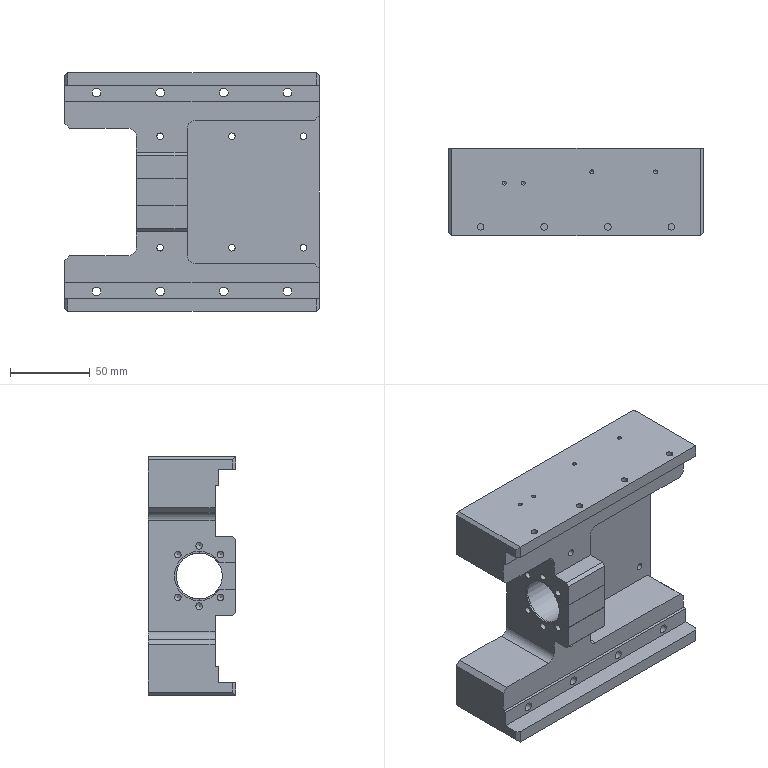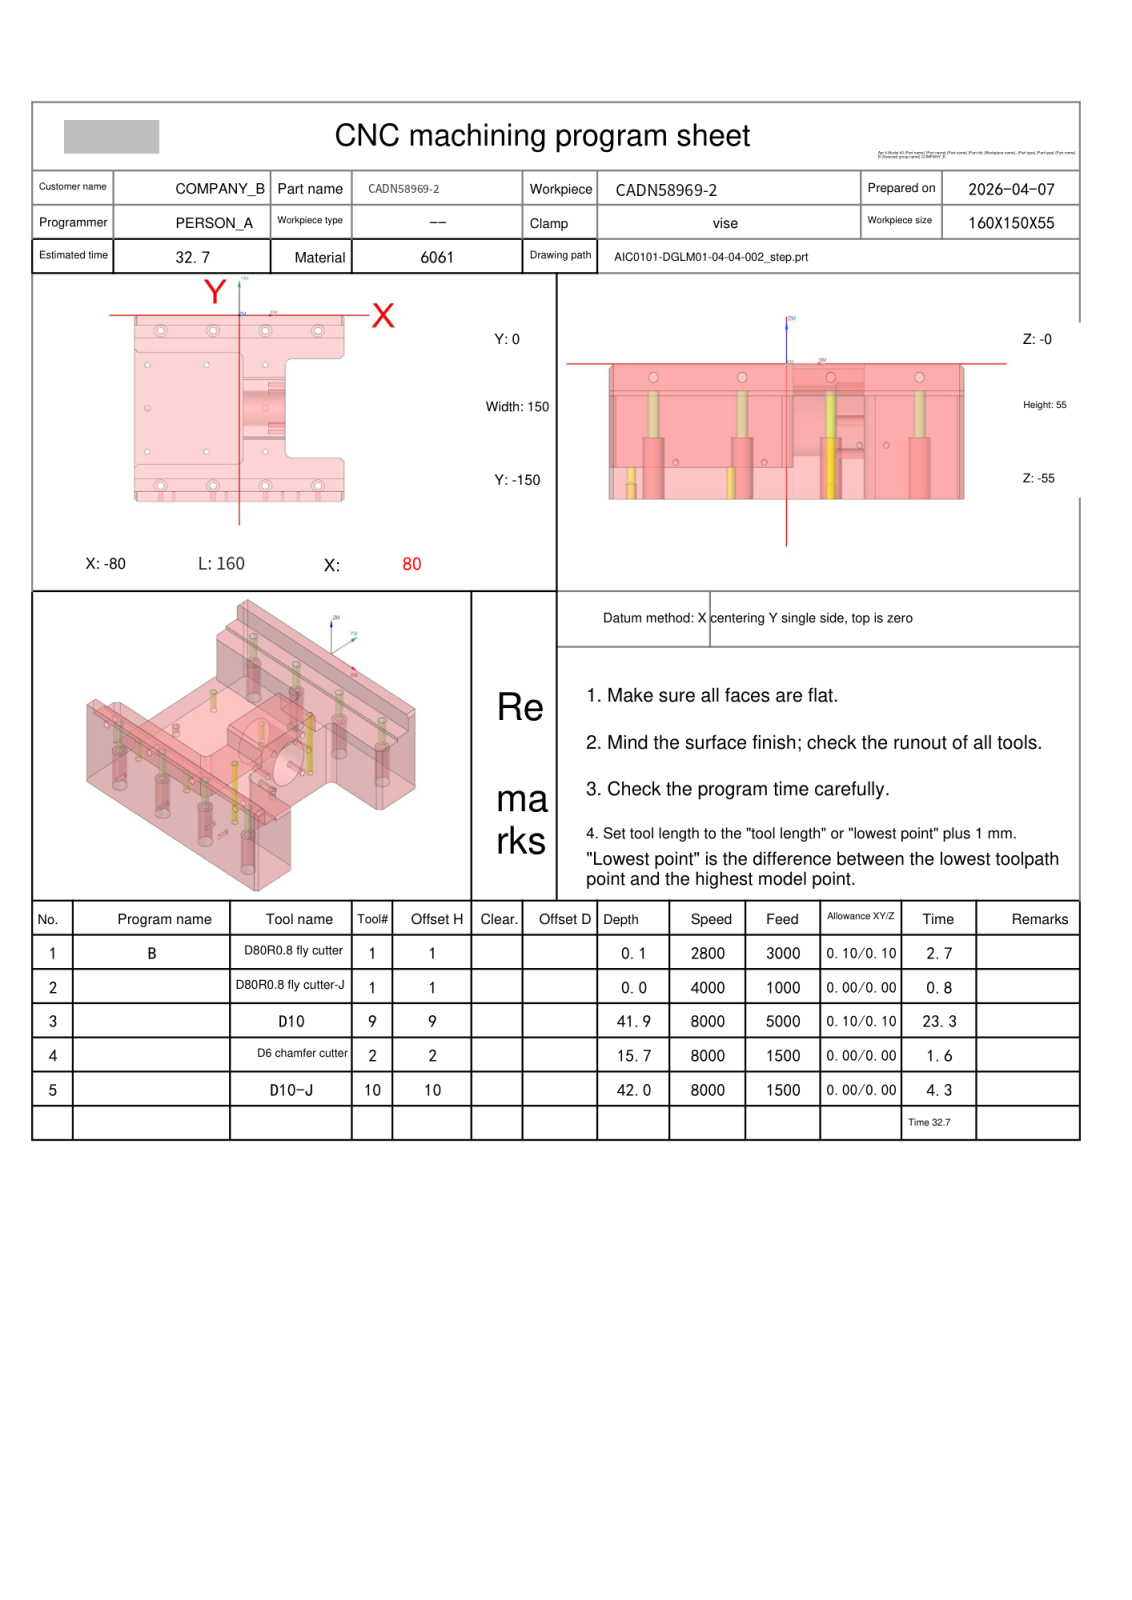NC program | NX | posted by the shop | part box 160 x 55 x 150 mm
Lines 209 to 1320 of 14160:
N3 T09 M06
(D10  D=10. R=0. H=09 ce=0.10 di=0.10)
G00 G90 G54 X-94.5 Y-82. M03 S8000
G43 H09 Z14.5
M08
Z.519
G01 Z-.681 F5000.
X-87.08
G03 X-80.08 Y-75. I0.0 J7.
G01 Y-34.166
X-80.147 Y-34.114
X-80.709 Y-33.618
X-83.001 Y-31.328
Y-29.888
X-80.08 Y-26.967
Y-23.302
X-80.079 Y-22.483
X-80.08 Y-14.353
Y-13.177
G02 X-84.225 Y-10.953 I.109 J5.178
X-85.158 Y-7.649 I5.387 J3.304
X-85.151 Y-7.349 I6.319 J0.0
G01 Y-2.
X-85.127 Y-1.943
X-83.936 Y-.752
X-83.823
Y-8.
G03 X-78.896 Y-13.096 I5.121 J.021
G01 X-78.343 Y-13.168
X-78.169 Y-13.178
X-77.979 Y-13.179
X75.306
X76.197
X77.98
X78.173 Y-13.178
X78.349 Y-13.168
X78.896 Y-13.096
G03 X83.823 Y-8. I-.194 J5.117
G01 Y-.752
X83.932
X85.127 Y-1.954
X85.151 Y-2.01
Y-7.353
X85.13 Y-8.246
G02 X80.08 Y-13.177 I-5.266 J.341
G01 X80.079 Y-22.483
X80.08 Y-23.302
Y-32.
X80.057 Y-32.057
X77.057 Y-35.057
X77. Y-35.08
X40.55
X39.665 Y-35.092
X38.787 Y-35.232
X37.908 Y-35.547
X37.587 Y-35.712
X37.278 Y-35.902
X37.033 Y-36.075
X36.639 Y-36.407
X36.282 Y-36.778
X36.156 Y-36.929
X35.9 Y-37.281
X35.677 Y-37.651
X35.305 Y-38.531
X35.181 Y-39.007
X35.116 Y-39.403
X35.08 Y-40.287
X35.084 Y-44.914
X35.08 Y-46.178
X35.001 Y-46.177
X35.
X34.999
X34.998
X34.92 Y-46.176
X3. Y-46.177
G03 X-2.096 Y-51.087 I.021 J-5.121
G01 X-2.136 Y-51.314
X-2.178 Y-51.857
X-2.179 Y-52.747
Y-97.253
X-2.178 Y-98.149
X-2.135 Y-98.694
X-2.096 Y-98.913
G03 X3. Y-103.823 I5.116 J.211
G01 X33.52
X34.92 Y-103.824
X34.999 Y-103.823
X35.
X35.001
X35.08
Y-105.099
Y-105.264
Y-109.713
X35.134 Y-111.033
X35.279 Y-111.384
X35.307 Y-111.478
X35.407 Y-111.94
X36.157 Y-113.073
X36.28 Y-113.22
X37.035 Y-113.926
X37.277 Y-114.098
X38.341 Y-114.696
X39.665 Y-114.908
X40.55 Y-114.92
X77.
X77.057 Y-114.943
X80.057 Y-117.943
X80.08 Y-118.
Y-121.92
Y-126.701
X80.079 Y-127.517
X80.08 Y-135.647
Y-136.824
G02 X82.733 Y-137.644 I-.158 J-5.213
X85.13 Y-141.758 I-2.811 J-4.393
G01 X85.151 Y-143.539
Y-148.
X85.127 Y-148.057
X83.936 Y-149.248
X83.823
X83.822 Y-141.973
G03 X78.898 Y-136.904 I-5.121 J-.048
G01 X78.343 Y-136.832
X78.169 Y-136.822
X-62.689 Y-136.821
X-77.088
X-77.534
X-77.775
X-78.015 Y-136.822
X-78.173
X-78.349 Y-136.832
X-78.897 Y-136.904
G03 X-83.823 Y-142. I.195 J-5.117
G01 Y-149.248
X-83.932
X-85.127 Y-148.046
X-85.151 Y-147.99
Y-143.538
X-85.13 Y-141.755
G02 X-80.08 Y-136.824 I5.207 J-.281
G01 Y-135.647
Y-123.032
X-83. Y-120.112
Y-118.672
X-80.706 Y-116.378
X-80.143 Y-115.882
X-80.08 Y-115.834
Y-78.014
G02 X-79.662 Y-77.201 I1. J-.001
G01 X-73.498 Y-72.799
G03 X-73.08 Y-71.986 I-.582 J.813
G01 Y-34.166
G03 X-73.83 Y-31.014 I-7. J0.0
G02 X-73.936 Y-30.566 I.894 J.448
X-73.83 Y-30.119 I1. J0.0
G03 X-73.08 Y-26.967 I-6.25 J3.152
G01 X-73.079 Y-21.176
G02 X-72.082 Y-20.179 I1. J-.003
G01 X32.086
G02 X32.78 Y-20.459 I0.0 J-1.
G01 X34.199 Y-21.826
G03 X34.678 Y-22.083 I.694 J.72
G02 X36.641 Y-24.525 I-.537 J-2.442
X34.822 Y-26.93 I-2.5 J0.0
G01 X27.87 Y-28.899
G02 X27.189 Y-28.994 I-.681 J2.405
X24.689 Y-26.494 I0.0 J2.5
X26.507 Y-24.088 I2.5 J0.0
G01 X32.238 Y-22.465
G03 X32.722 Y-22.157 I-.272 J.962
G01 X34.131 Y-20.525
G02 X34.888 Y-20.179 I.757 J-.654
G01 X72.082
G02 X73.079 Y-21.176 I-.003 J-1.
G01 Y-22.486
X73.08 Y-23.306
Y-27.083
G02 X72.083 Y-28.08 I-1. J.003
G01 X40.504
X39.062 Y-28.099
X37.038 Y-28.423
X35.112 Y-29.113
X34.153 Y-29.607
X33.422 Y-30.055
X32.748 Y-30.533
X31.851 Y-31.287
X31.063 Y-32.105
X30.632 Y-32.624
X30.061 Y-33.408
X29.423 Y-34.467
X28.658 Y-36.277
X28.325 Y-37.561
X28.197 Y-38.342
G02 X27.213 Y-39.177 I-.986 J.164
G01 X2.986
G03 X-9.055 Y-50.25 I.035 J-12.121
X-9.114 Y-50.767 I6.999 J-1.07
G01 X-9.156 Y-51.304
G03 X-9.178 Y-51.857 I7.058 J-.553
G01 Y-98.143
G03 X-9.156 Y-98.696 I7.08 J0.0
G01 X-9.114 Y-99.233
G03 X-9.055 Y-99.75 I7.058 J.553
X2.986 Y-110.823 I12.075 J1.048
G01 X27.176
G02 X28.168 Y-111.721 I-.003 J-1.
G03 X28.562 Y-113.441 I6.966 J.688
G01 X28.594 Y-113.549
G03 X29.573 Y-115.809 I6.813 J1.609
G01 X30.534 Y-117.258
X31.179 Y-118.034
X32.6 Y-119.362
X33.526 Y-120.019
X34.908 Y-120.797
G03 X37.234 Y-121.608 I3.433 J6.101
G01 X39.062 Y-121.901
X40.504 Y-121.92
X72.083
G02 X73.08 Y-122.917 I-.003 J-1.
G01 Y-126.696
X73.079 Y-127.514
Y-128.825
G02 X72.082 Y-129.822 I-1. J.003
G01 X34.936
G02 X34.18 Y-129.476 I0.0 J1.
G01 X32.765 Y-127.841
G03 X32.277 Y-127.532 I-.756 J-.654
G01 X26.504 Y-125.921
G02 X24.676 Y-123.513 I.672 J2.408
X27.176 Y-121.013 I2.5 J0.0
X27.848 Y-121.105 I0.0 J-2.5
G01 X34.849 Y-123.059
G02 X36.677 Y-125.467 I-.672 J-2.408
X34.725 Y-127.906 I-2.5 J0.0
G03 X34.249 Y-128.163 I.219 J-.976
G01 X32.823 Y-129.541
G02 X32.128 Y-129.822 I-.695 J.719
G01 X-72.083 Y-129.821
G02 X-73.08 Y-128.824 I.003 J1.
G01 Y-123.032
G03 X-73.83 Y-119.881 I-7. J0.0
G02 X-73.935 Y-119.433 I.894 J.448
X-73.83 Y-118.986 I1. J0.0
G03 X-73.08 Y-115.834 I-6.25 J3.152
G01 Y-78.014
G02 X-72.662 Y-77.201 I1. J0.0
G01 X-66.498 Y-72.799
G03 X-66.08 Y-71.986 I-.582 J.813
G01 Y-34.166
G03 X-66.49 Y-30.803 I-14. J0.0
G02 X-66.518 Y-30.566 I.972 J.237
X-66.49 Y-30.329 I1. J0.0
G03 X-66.126 Y-28.095 I-13.59 J3.363
G02 X-65.132 Y-27.179 I.996 J-.084
G01 X-11.561
G02 X-10.879 Y-27.448 I0.0 J-1.
G01 X-9.582 Y-28.658
G03 X-9.048 Y-28.915 I.682 J.731
G02 X-6.919 Y-31.388 I-.371 J-2.472
X-8.595 Y-33.748 I-2.5 J0.0
G01 X-14.748 Y-35.895
G02 X-15.572 Y-36.035 I-.824 J2.36
X-18.072 Y-33.535 I0.0 J2.5
X-16.396 Y-31.175 I2.5 J0.0
G01 X-11.377 Y-29.423
G03 X-10.938 Y-29.12 I-.329 J.944
G01 X-9.618 Y-27.538
G02 X-8.85 Y-27.179 I.768 J-.641
G01 X23.976
G02 X24.973 Y-28.179 I-.003 J-1.
X24.783 Y-28.765 I-1. J0.0
G01 X24.221 Y-29.535
X23.17 Y-31.283
X23.049 Y-31.57
G02 X22.132 Y-32.177 I-.92 J.393
G01 X2.976
G03 X-16.009 Y-49.431 I.045 J-19.121
X-16.093 Y-50.22 I13.953 J-1.889
G01 X-16.135 Y-50.757
G03 X-16.178 Y-51.857 I14.037 J-1.1
G01 Y-98.143
G03 X-16.135 Y-99.243 I14.08 J0.0
G01 X-16.093 Y-99.78
G03 X-16.009 Y-100.569 I14.037 J1.1
X2.976 Y-117.823 I19.029 J1.867
G01 X22.082
G02 X22.966 Y-118.361 I-.003 J-1.
G03 X23.739 Y-119.678 I12.441 J6.421
G01 X24.796 Y-121.272
G02 X24.961 Y-121.822 I-.835 J-.55
X23.964 Y-122.822 I-1. J0.0
G01 X-8.85
G02 X-9.618 Y-122.462 I0.0 J1.
G01 X-10.938 Y-120.88
G03 X-11.376 Y-120.577 I-.768 J-.641
G01 X-16.395 Y-118.826
G02 X-18.072 Y-116.465 I.824 J2.36
X-15.572 Y-113.965 I2.5 J0.0
X-14.748 Y-114.105 I0.0 J-2.5
G01 X-8.595 Y-116.252
G02 X-6.919 Y-118.612 I-.824 J-2.36
X-9.048 Y-121.085 I-2.5 J0.0
G03 X-9.582 Y-121.343 I.148 J-.989
G01 X-10.879 Y-122.553
G02 X-11.561 Y-122.822 I-.682 J.731
G01 X-65.132 Y-122.821
G02 X-66.125 Y-121.905 I.003 J1.
G03 X-66.49 Y-119.67 I-13.955 J-1.127
G02 X-66.518 Y-119.433 I.972 J.237
X-66.49 Y-119.196 I1. J0.0
G03 X-66.08 Y-115.834 I-13.59 J3.362
G01 Y-115.821
Y-78.014
G02 X-65.662 Y-77.201 I1. J0.0
G01 X-59.498 Y-72.799
G03 X-59.08 Y-71.986 I-.582 J.813
G01 Y-35.175
G02 X-58.084 Y-34.179 I1. J-.004
G01 X-18.786
G02 X-17.79 Y-35.179 I-.004 J-1.
X-17.984 Y-35.77 I-1. J0.0
G03 X-22.963 Y-48.623 I21.004 J-15.528
X-23.071 Y-49.672 I20.907 J-2.697
G01 X-23.114 Y-50.21
G03 X-23.178 Y-51.857 I21.016 J-1.647
G01 Y-98.143
G03 X-23.114 Y-99.79 I21.08 J0.0
G01 X-23.071 Y-100.327
G03 X-22.963 Y-101.377 I21.016 J1.647
X-17.983 Y-114.23 I25.983 J2.675
G02 X-17.79 Y-114.822 I-.806 J-.592
X-18.786 Y-115.822 I-1. J0.0
G01 X-58.084 Y-115.821
G02 X-59.08 Y-114.825 I.004 J1.
G01 Y-78.014
G02 X-58.662 Y-77.201 I1. J0.0
G01 X-52.498 Y-72.799
G03 X-52.08 Y-71.986 I-.582 J.813
G01 Y-42.175
G02 X-51.084 Y-41.179 I1. J-.004
G01 X-29.855
G02 X-28.859 Y-42.179 I-.004 J-1.
X-28.894 Y-42.442 I-1. J0.0
G03 X-29.917 Y-47.817 I31.915 J-8.856
X-30.05 Y-49.125 I27.861 J-3.503
G01 X-30.092 Y-49.663
G03 X-30.178 Y-51.857 I27.994 J-2.194
G01 Y-98.143
G03 X-30.092 Y-100.337 I28.08 J0.0
G01 X-30.05 Y-100.874
G03 X-29.917 Y-102.183 I27.994 J2.195
X-28.894 Y-107.558 I32.937 J3.481
G02 X-28.859 Y-107.822 I-.965 J-.264
X-29.855 Y-108.822 I-1. J0.0
G01 X-51.084 Y-108.821
G02 X-52.08 Y-107.825 I.004 J1.
G01 Y-78.014
G02 X-51.662 Y-77.201 I1. J0.0
G01 X-45.498 Y-72.799
G03 X-45.08 Y-71.986 I-.582 J.813
G01 Y-49.175
G02 X-44.084 Y-48.179 I1. J-.004
G01 X-38.074
G02 X-37.078 Y-49.179 I-.004 J-1.
G01 X-37.081 Y-49.249
G03 X-37.178 Y-51.857 I34.983 J-2.608
G01 Y-98.143
G03 X-37.081 Y-100.751 I35.08 J0.0
G01 X-37.078 Y-100.821
G02 X-38.074 Y-101.821 I-1. J0.0
G01 X-44.084
G02 X-45.08 Y-100.825 I.004 J1.
G01 Y-75.
Y-74.5
G03 X-52.08 Y-67.5 I-7. J0.0
G01 Z.519
G00 Z3.
G01 X-94.5 Y-82. F6000.
G00 Z-.163
G01 Z-1.363 F5000.
X-87.08
G03 X-80.08 Y-75. I0.0 J7.
G01 Y-34.166
X-80.147 Y-34.114
X-80.709 Y-33.618
X-83.001 Y-31.328
Y-29.888
X-80.08 Y-26.967
Y-23.302
X-80.079 Y-22.483
X-80.08 Y-13.177
G02 X-82.321 Y-12.615 I.109 J5.178
X-84.225 Y-10.953 I2.35 J4.615
X-85.158 Y-7.649 I5.387 J3.304
X-85.151 Y-7.349 I6.319 J0.0
G01 Y-2.
X-85.127 Y-1.943
X-84.617 Y-1.433
X-84.504
Y-8.
G03 X-79.383 Y-13.1 I5.121 J.021
G01 X-79.362
X-78.877
X-78.343 Y-13.168
X-78.169 Y-13.178
X-77.979 Y-13.179
X75.306
X76.197
X77.98
X78.173 Y-13.178
X78.349 Y-13.168
X78.877 Y-13.1
X79.362
X79.383
G03 X84.504 Y-8. I0.0 J5.121
G01 Y-1.433
X84.61
X85.127 Y-1.954
X85.151 Y-2.01
Y-7.353
X85.13 Y-8.246
G02 X83. Y-12.149 I-5.266 J.341
X80.08 Y-13.177 I-3.136 J4.244
G01 X80.079 Y-22.483
X80.08 Y-23.302
Y-32.
X80.057 Y-32.057
X77.057 Y-35.057
X77. Y-35.08
X40.55
X39.665 Y-35.092
X38.787 Y-35.232
X37.908 Y-35.547
X37.587 Y-35.712
X37.278 Y-35.902
X37.033 Y-36.075
X36.639 Y-36.407
X36.282 Y-36.778
X36.156 Y-36.929
X35.9 Y-37.281
X35.677 Y-37.651
X35.305 Y-38.531
X35.181 Y-39.007
X35.116 Y-39.403
X35.08 Y-40.287
X35.084 Y-44.914
X35.083 Y-45.496
X35.003
Y-45.495
X34.994 Y-45.496
X34.923 Y-45.495
X3. Y-45.496
G03 X-2.1 Y-50.617 I.021 J-5.121
G01 Y-50.638
Y-51.111
X-2.136 Y-51.314
X-2.178 Y-51.857
X-2.179 Y-52.747
Y-97.253
X-2.178 Y-98.149
X-2.135 Y-98.694
X-2.1 Y-98.889
Y-99.387
G03 X3. Y-104.504 I5.121 J.004
G01 X34.92
X34.999
X35. Y-104.505
X35.001 Y-104.504
X35.08
Y-105.099
Y-105.264
Y-109.713
X35.134 Y-111.033
X35.279 Y-111.384
X35.312 Y-111.504
X35.407 Y-111.94
X36.157 Y-113.073
X36.28 Y-113.22
X37.035 Y-113.926
X37.277 Y-114.098
X38.341 Y-114.696
X39.665 Y-114.908
X40.55 Y-114.92
X77.
X77.057 Y-114.943
X80.057 Y-117.943
X80.08 Y-118.
Y-121.92
Y-126.701
X80.079 Y-127.517
X80.08 Y-136.824
G02 X85.13 Y-141.758 I-.158 J-5.213
G01 X85.151 Y-143.539
Y-148.
X85.127 Y-148.057
X84.617 Y-148.567
X84.504
Y-142.
G03 X79.383 Y-136.9 I-5.121 J-.021
G01 X79.362
X78.879
X78.343 Y-136.832
X78.169 Y-136.822
X-62.689 Y-136.821
X-77.088
X-77.534
X-78.015 Y-136.822
X-78.173
X-78.349 Y-136.832
X-78.879 Y-136.9
X-79.362
X-79.383
G03 X-84.504 Y-142. I0.0 J-5.121
G01 Y-148.567
X-84.61
X-85.127 Y-148.046
X-85.151 Y-147.99
Y-143.538
X-85.13 Y-141.755
G02 X-80.08 Y-136.824 I5.207 J-.281
G01 Y-123.032
X-83. Y-120.112
Y-118.672
X-80.706 Y-116.378
X-80.143 Y-115.882
X-80.08 Y-115.834
Y-78.014
G02 X-79.662 Y-77.201 I1. J0.0
G01 X-73.498 Y-72.799
G03 X-73.08 Y-71.986 I-.582 J.813
G01 Y-34.166
G03 X-73.83 Y-31.014 I-7. J0.0
G02 X-73.936 Y-30.566 I.894 J.447
X-73.83 Y-30.119 I1. J0.0
G03 X-73.08 Y-26.967 I-6.25 J3.152
G01 X-73.079 Y-21.176
G02 X-72.082 Y-20.179 I1. J-.003
G01 X32.086
G02 X32.78 Y-20.459 I0.0 J-1.
G01 X34.199 Y-21.826
G03 X34.678 Y-22.083 I.694 J.72
G02 X36.641 Y-24.525 I-.537 J-2.442
X34.822 Y-26.93 I-2.5 J0.0
G01 X27.87 Y-28.899
G02 X27.189 Y-28.994 I-.681 J2.405
X24.689 Y-26.494 I0.0 J2.5
X26.507 Y-24.088 I2.5 J0.0
G01 X32.238 Y-22.465
G03 X32.722 Y-22.157 I-.272 J.962
G01 X34.131 Y-20.525
G02 X34.888 Y-20.179 I.757 J-.654
G01 X72.082
G02 X73.079 Y-21.176 I-.003 J-1.
G01 Y-22.486
X73.08 Y-23.306
Y-27.083
G02 X72.083 Y-28.08 I-1. J.003
G01 X40.504
X39.062 Y-28.099
X37.038 Y-28.423
X35.112 Y-29.113
X34.153 Y-29.607
X33.422 Y-30.055
X32.748 Y-30.533
X31.851 Y-31.287
X31.063 Y-32.105
X30.632 Y-32.624
X30.061 Y-33.408
X29.423 Y-34.467
X28.658 Y-36.277
X28.325 Y-37.561
X28.309 Y-37.661
G02 X27.325 Y-38.496 I-.986 J.165
G01 X2.986
G03 X-9.1 Y-50.608 I.035 J-12.121
G01 X-9.156 Y-51.303
G03 X-9.178 Y-51.857 I7.058 J-.553
G01 Y-98.143
G03 X-9.156 Y-98.697 I7.08 J0.0
G01 X-9.1 Y-99.392
G03 X2.986 Y-111.504 I12.121 J.009
G01 X27.274
G02 X28.253 Y-112.317 I-.003 J-1.
G03 X28.562 Y-113.441 I6.881 J1.284
G01 X28.594 Y-113.549
G03 X29.573 Y-115.809 I6.813 J1.609
G01 X30.534 Y-117.258
X31.179 Y-118.034
X32.6 Y-119.362
X33.526 Y-120.019
X34.908 Y-120.797
G03 X37.234 Y-121.608 I3.433 J6.101
G01 X39.062 Y-121.901
X40.504 Y-121.92
X72.083
G02 X73.08 Y-122.917 I-.003 J-1.
G01 Y-126.696
X73.079 Y-127.514
Y-128.825
G02 X72.082 Y-129.822 I-1. J.003
G01 X34.936
G02 X34.18 Y-129.476 I0.0 J1.
G01 X32.765 Y-127.841
G03 X32.277 Y-127.532 I-.756 J-.654
G01 X26.504 Y-125.921
G02 X24.676 Y-123.513 I.672 J2.408
X27.176 Y-121.013 I2.5 J0.0
X27.848 Y-121.105 I0.0 J-2.5
G01 X34.849 Y-123.059
G02 X36.677 Y-125.467 I-.672 J-2.408
X34.725 Y-127.906 I-2.5 J0.0
G03 X34.249 Y-128.163 I.219 J-.976
G01 X32.822 Y-129.541
G02 X32.128 Y-129.822 I-.695 J.719
G01 X-62.689 Y-129.821
X-72.083
G02 X-73.08 Y-128.824 I.003 J1.
G01 Y-123.032
G03 X-73.83 Y-119.881 I-7. J0.0
G02 X-73.935 Y-119.433 I.894 J.447
X-73.83 Y-118.986 I1. J0.0
G03 X-73.08 Y-115.834 I-6.25 J3.152
G01 Y-78.014
G02 X-72.662 Y-77.201 I1. J0.0
G01 X-66.498 Y-72.799
G03 X-66.08 Y-71.986 I-.582 J.813
G01 Y-34.166
G03 X-66.49 Y-30.803 I-14. J0.0
G02 X-66.518 Y-30.566 I.972 J.237
X-66.49 Y-30.33 I1. J0.0
G03 X-66.125 Y-28.094 I-13.59 J3.363
G02 X-65.133 Y-27.179 I.996 J-.084
G01 X-12.45
G02 X-11.771 Y-27.444 I0.0 J-1.
G01 X-10.51 Y-28.609
G03 X-9.96 Y-28.866 I.679 J.735
G02 X-7.78 Y-31.346 I-.32 J-2.479
X-9.412 Y-33.691 I-2.5 J0.0
G01 X-15.215 Y-35.837
G02 X-16.082 Y-35.992 I-.867 J2.345
X-18.582 Y-33.492 I0.0 J2.5
X-16.95 Y-31.148 I2.5 J0.0
G01 X-12.254 Y-29.411
G03 X-11.83 Y-29.11 I-.347 J.938
G01 X-10.536 Y-27.542
G02 X-9.765 Y-27.179 I.771 J-.637
G01 X23.976
G02 X24.973 Y-28.179 I-.004 J-1.
X24.783 Y-28.765 I-1. J0.0
G01 X24.221 Y-29.535
X23.332 Y-31.014
G02 X22.48 Y-31.496 I-.855 J.518
G01 X2.976
G03 X-16.097 Y-50.29 I.045 J-19.121
G01 X-16.134 Y-50.747
G03 X-16.178 Y-51.856 I14.036 J-1.11
G01 Y-98.144
G03 X-16.134 Y-99.253 I14.08 J0.0
G01 X-16.097 Y-99.71
G03 X2.976 Y-118.504 I19.118 J.326
G01 X22.457
G02 X23.315 Y-118.997 I-.004 J-1.
G03 X23.739 Y-119.678 I12.092 J7.056
G01 X24.796 Y-121.272
G02 X24.961 Y-121.822 I-.835 J-.55
X23.965 Y-122.822 I-1. J0.0
G01 X-9.765 Y-122.821
G02 X-10.536 Y-122.458 I0.0 J1.
G01 X-11.83 Y-120.89
G03 X-12.254 Y-120.589 I-.771 J-.637
G01 X-16.95 Y-118.852
G02 X-18.582 Y-116.508 I.867 J2.345
X-16.082 Y-114.008 I2.5 J0.0
X-15.215 Y-114.163 I0.0 J-2.5
G01 X-9.412 Y-116.309
G02 X-7.78 Y-118.654 I-.867 J-2.345
X-9.96 Y-121.134 I-2.5 J0.0
G03 X-10.511 Y-121.391 I.128 J-.992
G01 X-11.771 Y-122.556
G02 X-12.45 Y-122.821 I-.679 J.734
G01 X-62.689
X-65.132
G02 X-66.125 Y-121.905 I.003 J1.
G03 X-66.49 Y-119.67 I-13.955 J-1.127
G02 X-66.518 Y-119.433 I.972 J.237
X-66.49 Y-119.197 I1. J0.0
G03 X-66.08 Y-115.834 I-13.59 J3.362
G01 Y-115.821
Y-78.014
G02 X-65.662 Y-77.201 I1. J0.0
G01 X-59.498 Y-72.799
G03 X-59.08 Y-71.986 I-.582 J.813
G01 Y-35.175
G02 X-58.084 Y-34.179 I1. J-.004
G01 X-19.273
G02 X-18.277 Y-35.179 I-.004 J-1.
X-18.453 Y-35.745 I-1. J0.0
G03 X-23.091 Y-49.93 I21.474 J-14.872
G01 X-23.112 Y-50.189
G03 X-23.178 Y-51.856 I21.014 J-1.668
G01 Y-98.144
G03 X-23.112 Y-99.811 I21.08 J.001
G01 X-23.091 Y-100.07
G03 X-18.453 Y-114.255 I26.112 J.686
G02 X-18.277 Y-114.821 I-.824 J-.566
X-19.273 Y-115.821 I-1. J0.0
G01 X-58.084
G02 X-59.08 Y-114.825 I.004 J1.
G01 Y-78.014
G02 X-58.662 Y-77.201 I1. J0.0
G01 X-52.498 Y-72.799
G03 X-52.08 Y-71.986 I-.582 J.813
G01 Y-42.175
G02 X-51.084 Y-41.179 I1. J-.004
G01 X-30.036
G02 X-29.04 Y-42.179 I-.004 J-1.
X-29.07 Y-42.422 I-1. J0.0
G03 X-30.083 Y-49.544 I32.091 J-8.195
G01 X-30.09 Y-49.63
G03 X-30.178 Y-51.856 I27.992 J-2.227
G01 Y-98.144
G03 X-30.083 Y-100.456 I28.08 J.001
X-29.07 Y-107.578 I33.103 J1.072
G02 X-29.04 Y-107.821 I-.97 J-.243
X-30.036 Y-108.821 I-1. J0.0
G01 X-51.084
G02 X-52.08 Y-107.825 I.004 J1.
G01 Y-78.014
G02 X-51.662 Y-77.201 I1. J0.0
G01 X-45.498 Y-72.799
G03 X-45.08 Y-71.986 I-.582 J.813
G01 Y-49.174
G02 X-44.084 Y-48.179 I1. J-.004
G01 X-38.074
G02 X-37.078 Y-49.179 I-.004 J-1.
G01 X-37.081 Y-49.249
G03 X-37.178 Y-51.856 I34.983 J-2.608
G01 Y-98.144
G03 X-37.081 Y-100.751 I35.08 J.001
G01 X-37.079 Y-100.821
G02 X-38.074 Y-101.821 I-1. J0.0
G01 X-44.084
G02 X-45.08 Y-100.825 I.004 J1.
G01 Y-75.
Y-74.5
G03 X-52.08 Y-67.5 I-7. J0.0
G01 Z-.163
G00 Z3.
G01 X-94.5 Y-82. F6000.
G00 Z-.844
G01 Z-2.044 F5000.
X-87.08
G03 X-80.08 Y-75. I0.0 J7.
G01 Y-34.166
X-80.147 Y-34.114
X-80.709 Y-33.618
X-83.001 Y-31.328
Y-29.888
X-80.08 Y-26.967
Y-23.302
X-80.079 Y-22.483
X-80.08 Y-13.177
X-80.059 Y-13.1
X-79.362
X-78.877
X-78.343 Y-13.168
X-78.169 Y-13.178
X-77.979 Y-13.179
X75.306
X76.197
X77.98
X78.173 Y-13.178
X78.349 Y-13.168
X78.877 Y-13.1
X79.404
X80.07
X80.08 Y-13.177
X80.079 Y-22.483
X80.08 Y-23.302
Y-32.
X80.057 Y-32.057
X77.057 Y-35.057
X77. Y-35.08
X40.55
X39.665 Y-35.092
X38.787 Y-35.232
X37.908 Y-35.547
X37.587 Y-35.712
X37.278 Y-35.902
X37.033 Y-36.075
X36.639 Y-36.407
X36.282 Y-36.778
X36.156 Y-36.929
X35.9 Y-37.281
X35.677 Y-37.651
X35.305 Y-38.531
X35.181 Y-39.007
X35.116 Y-39.403
X35.08 Y-40.287
X35.081 Y-44.889
X35.023 Y-44.9
X35.022 Y-44.899
X26.424 Y-44.9
X3.
G03 X-2.1 Y-50. I0.0 J-5.1
G01 Y-51.111
X-2.136 Y-51.314
X-2.178 Y-51.857
X-2.179 Y-52.747
Y-97.253
X-2.178 Y-98.149
X-2.135 Y-98.694
X-2.1 Y-98.889
Y-99.404
Y-100.045
G03 X3. Y-105.1 I5.1 J.045
G01 X34.92
X35.08
Y-105.264
Y-109.713
X35.134 Y-111.033
X35.279 Y-111.384
X35.307 Y-111.478
X35.407 Y-111.94
X36.157 Y-113.073
X36.28 Y-113.22
X37.035 Y-113.926
X37.277 Y-114.098
X38.341 Y-114.696
X39.665 Y-114.908
X40.55 Y-114.92
X77.
X77.057 Y-114.943
X80.057 Y-117.943
X80.08 Y-118.
Y-121.92
Y-126.701
X80.079 Y-127.517
X80.08 Y-136.824
X79.92 Y-136.899
X78.879 Y-136.9
X78.867 Y-136.898
X78.559 Y-136.859
X78.343 Y-136.832
X78.169 Y-136.822
X-62.689 Y-136.821
X-77.088
X-77.311
X-77.534
X-78.173 Y-136.822
X-78.349 Y-136.832
X-78.879 Y-136.9
X-79.363
X-79.404
X-79.92
X-80.08 Y-136.824
Y-123.032
X-83. Y-120.112
Y-118.672
X-80.706 Y-116.378
X-80.143 Y-115.882
X-80.08 Y-115.834
Y-78.014
G02 X-79.662 Y-77.201 I1. J0.0
G01 X-73.498 Y-72.799
G03 X-73.08 Y-71.986 I-.582 J.813
G01 Y-34.166
G03 X-73.83 Y-31.014 I-7. J0.0
G02 X-73.936 Y-30.566 I.894 J.447
X-73.83 Y-30.119 I1. J0.0
G03 X-73.08 Y-26.967 I-6.25 J3.152
G01 X-73.079 Y-21.175
G02 X-72.083 Y-20.179 I1. J-.003
G01 X32.086
G02 X32.78 Y-20.459 I0.0 J-1.
G01 X34.199 Y-21.826
G03 X34.678 Y-22.083 I.694 J.72
G02 X36.641 Y-24.525 I-.537 J-2.442
X34.822 Y-26.93 I-2.5 J0.0
G01 X27.87 Y-28.899
G02 X27.189 Y-28.994 I-.681 J2.405
X24.689 Y-26.494 I0.0 J2.5
X26.507 Y-24.088 I2.5 J0.0
G01 X32.238 Y-22.465
G03 X32.722 Y-22.157 I-.272 J.962
G01 X34.131 Y-20.525
G02 X34.888 Y-20.179 I.757 J-.654
G01 X72.083
G02 X73.079 Y-21.175 I-.003 J-1.
G01 Y-22.486
X73.08 Y-23.306
Y-27.083
G02 X72.083 Y-28.08 I-1. J.003
G01 X40.504
X39.062 Y-28.099
X37.038 Y-28.423
X35.112 Y-29.113
X34.153 Y-29.607
X33.422 Y-30.055
X32.748 Y-30.533
X31.851 Y-31.287
X31.063 Y-32.105
X30.632 Y-32.624
X30.061 Y-33.408
X29.423 Y-34.467
X28.658 Y-36.277
X28.43 Y-37.154
G02 X27.466 Y-37.9 I-.967 J.254
G01 X3.
G03 X-9.1 Y-50. I0.0 J-12.1
G01 X-9.104 Y-50.65
X-9.167 Y-51.456
G03 X-9.179 Y-51.868 I7.069 J-.413
G01 X-9.178 Y-51.966
X-9.179 Y-52.744
Y-97.256
X-9.178 Y-98.143
G03 X-9.156 Y-98.696 I7.08 J0.0
G01 X-9.1 Y-100.106
G03 X3. Y-112.1 I12.1 J.106
G01 X27.409
G02 X28.371 Y-112.839 I-.003 J-1.
G03 X28.562 Y-113.441 I6.763 J1.805
G01 X28.594 Y-113.549
G03 X29.573 Y-115.809 I6.813 J1.608
G01 X30.534 Y-117.258
X31.179 Y-118.034
X32.6 Y-119.362
X33.526 Y-120.019
X34.908 Y-120.797
G03 X37.234 Y-121.608 I3.433 J6.101
G01 X39.062 Y-121.901
X40.504 Y-121.92
X72.083
G02 X73.08 Y-122.917 I-.003 J-1.
G01 Y-126.696
X73.079 Y-127.514
Y-128.825
G02 X72.082 Y-129.822 I-1. J.003
G01 X34.936
G02 X34.18 Y-129.476 I0.0 J1.
G01 X32.765 Y-127.841
G03 X32.277 Y-127.532 I-.756 J-.654
G01 X26.504 Y-125.921
G02 X24.676 Y-123.513 I.672 J2.408
X27.176 Y-121.013 I2.5 J0.0
X27.848 Y-121.105 I0.0 J-2.5
G01 X34.849 Y-123.059
G02 X36.677 Y-125.467 I-.672 J-2.408
X34.725 Y-127.906 I-2.5 J0.0
G03 X34.249 Y-128.163 I.219 J-.976
G01 X32.822 Y-129.541
G02 X32.128 Y-129.822 I-.695 J.719
G01 X-62.689 Y-129.821
X-72.083
G02 X-73.08 Y-128.824 I.003 J1.
G01 Y-123.032
G03 X-73.83 Y-119.881 I-7. J0.0
G02 X-73.935 Y-119.433 I.894 J.447
X-73.83 Y-118.986 I1. J0.0
G03 X-73.08 Y-115.834 I-6.25 J3.152
G01 Y-78.014
G02 X-72.662 Y-77.201 I1. J0.0
G01 X-66.498 Y-72.799
G03 X-66.08 Y-71.986 I-.582 J.813
G01 Y-34.166
G03 X-66.49 Y-30.803 I-14. J0.0
G02 X-66.518 Y-30.566 I.972 J.237
X-66.49 Y-30.33 I1. J0.0
G03 X-66.125 Y-28.094 I-13.59 J3.363
G02 X-65.133 Y-27.179 I.996 J-.084
G01 X-13.18
G02 X-12.504 Y-27.441 I0.0 J-1.
G01 X-11.274 Y-28.569
G03 X-10.709 Y-28.826 I.676 J.737
G02 X-8.486 Y-31.311 I-.277 J-2.485
X-10.082 Y-33.641 I-2.5 J0.0
G01 X-15.61 Y-35.786
G02 X-16.514 Y-35.955 I-.904 J2.331
X-19.014 Y-33.455 I0.0 J2.5
X-17.418 Y-31.124 I2.5 J0.0
G01 X-12.976 Y-29.401
G03 X-12.563 Y-29.102 I-.362 J.932
G01 X-11.29 Y-27.545
G02 X-10.516 Y-27.179 I.774 J-.633
G01 X23.976
G02 X24.973 Y-28.179 I-.004 J-1.
X24.783 Y-28.765 I-1. J0.0
G01 X24.221 Y-29.535
X23.69 Y-30.419
G02 X22.839 Y-30.9 I-.855 J.518
G01 X3.
G03 X-16.1 Y-50. I0.0 J-19.1
G01 X-16.155 Y-51.059
G03 X-16.178 Y-51.863 I14.057 J-.804
G01 Y-51.963
X-16.179 Y-52.742
Y-97.258
X-16.178 Y-98.037
Y-98.138
G03 X-16.146 Y-99.088 I14.08 J0.0
G01 X-16.098 Y-100.29
G03 X3. Y-119.1 I19.098 J.29
G01 X22.824
G02 X23.657 Y-119.553 I-.004 J-1.
G01 X23.739 Y-119.678
X24.796 Y-121.272
G02 X24.961 Y-121.822 I-.835 J-.55
X23.965 Y-122.822 I-1. J0.0
G01 X-10.516 Y-122.821
G02 X-11.29 Y-122.455 I0.0 J1.
G01 X-12.563 Y-120.898
G03 X-12.975 Y-120.599 I-.774 J-.633
G01 X-17.418 Y-118.876
G02 X-19.014 Y-116.545 I.904 J2.331
X-16.514 Y-114.045 I2.5 J0.0
X-15.61 Y-114.214 I0.0 J-2.5
G01 X-10.082 Y-116.359
G02 X-8.486 Y-118.689 I-.904 J-2.331
X-10.709 Y-121.174 I-2.5 J0.0
G03 X-11.274 Y-121.431 I.111 J-.994
G01 X-12.504 Y-122.559
G02 X-13.18 Y-122.821 I-.676 J.737
G01 X-62.689
X-65.133
G02 X-66.125 Y-121.905 I.004 J1.
G03 X-66.49 Y-119.67 I-13.955 J-1.127
G02 X-66.518 Y-119.433 I.972 J.237
X-66.49 Y-119.197 I1. J0.0
G03 X-66.08 Y-115.834 I-13.59 J3.363
G01 Y-115.821
Y-78.014
G02 X-65.662 Y-77.201 I1. J0.0
G01 X-59.498 Y-72.799
G03 X-59.08 Y-71.986 I-.582 J.813
G01 Y-35.175
G02 X-58.084 Y-34.179 I1. J-.004
G01 X-19.684
G02 X-18.688 Y-35.179 I-.004 J-1.
X-18.848 Y-35.722 I-1. J0.0
G03 X-23.099 Y-49.803 I21.848 J-14.278
G01 X-23.145 Y-50.678
G03 X-23.178 Y-51.863 I21.047 J-1.185
G01 Y-51.983
X-23.179 Y-52.739
Y-97.261
X-23.178 Y-98.017
Y-98.138
G03 X-23.137 Y-99.456 I21.08 J0.0
G01 X-23.095 Y-100.492
G03 X-18.848 Y-114.278 I26.095 J.492
G02 X-18.688 Y-114.821 I-.839 J-.544
X-19.684 Y-115.821 I-1. J0.0
G01 X-58.084
G02 X-59.08 Y-114.825 I.004 J1.
G01 Y-78.014
G02 X-58.662 Y-77.201 I1. J0.0
G01 X-52.498 Y-72.799
G03 X-52.08 Y-71.986 I-.582 J.813
G01 Y-42.174
G02 X-51.084 Y-41.179 I1. J-.004
G01 X-30.187
G02 X-29.191 Y-42.179 I-.004 J-1.
X-29.217 Y-42.404 I-1. J0.0
G03 X-30.097 Y-49.584 I32.217 J-7.596
G01 X-30.135 Y-50.299
G03 X-30.178 Y-51.863 I28.036 J-1.564
G01 Y-51.998
X-30.179 Y-52.737
Y-97.263
X-30.178 Y-98.001
Y-98.138
G03 X-30.129 Y-99.811 I28.08 J0.0
G01 X-30.093 Y-100.703
G03 X-29.217 Y-107.596 I33.093 J.703
G02 X-29.191 Y-107.821 I-.974 J-.225
X-30.187 Y-108.821 I-1. J0.0
G01 X-51.084
G02 X-52.08 Y-107.825 I.004 J1.
G01 Y-78.014
G02 X-51.662 Y-77.201 I1. J0.0
G01 X-45.498 Y-72.799
G03 X-45.08 Y-71.986 I-.582 J.813
G01 Y-49.174
G02 X-44.084 Y-48.179 I1. J-.004
G01 X-38.087
G02 X-37.092 Y-49.179 I-.004 J-1.
G01 Y-49.194
X-37.095 Y-49.35
X-37.125 Y-49.922
G03 X-37.178 Y-51.863 I35.026 J-1.941
G01 Y-52.012
X-37.179 Y-52.734
Y-97.265
X-37.178 Y-97.988
Y-98.138
G03 X-37.12 Y-100.157 I35.08 J0.0
G01 X-37.095 Y-100.785
X-37.094 Y-100.821
G02 X-38.09 Y-101.821 I-1. J0.0
G01 X-44.084
G02 X-45.08 Y-100.826 I.004 J1.
G01 Y-75.
Y-74.5
G03 X-52.08 Y-67.5 I-7. J0.0
G01 Z-.844
G00 Z3.
G01 X-94.5 Y-82. F6000.
G00 Z-1.525
G01 Z-2.725 F5000.
X-87.08
G03 X-80.08 Y-75. I0.0 J7.